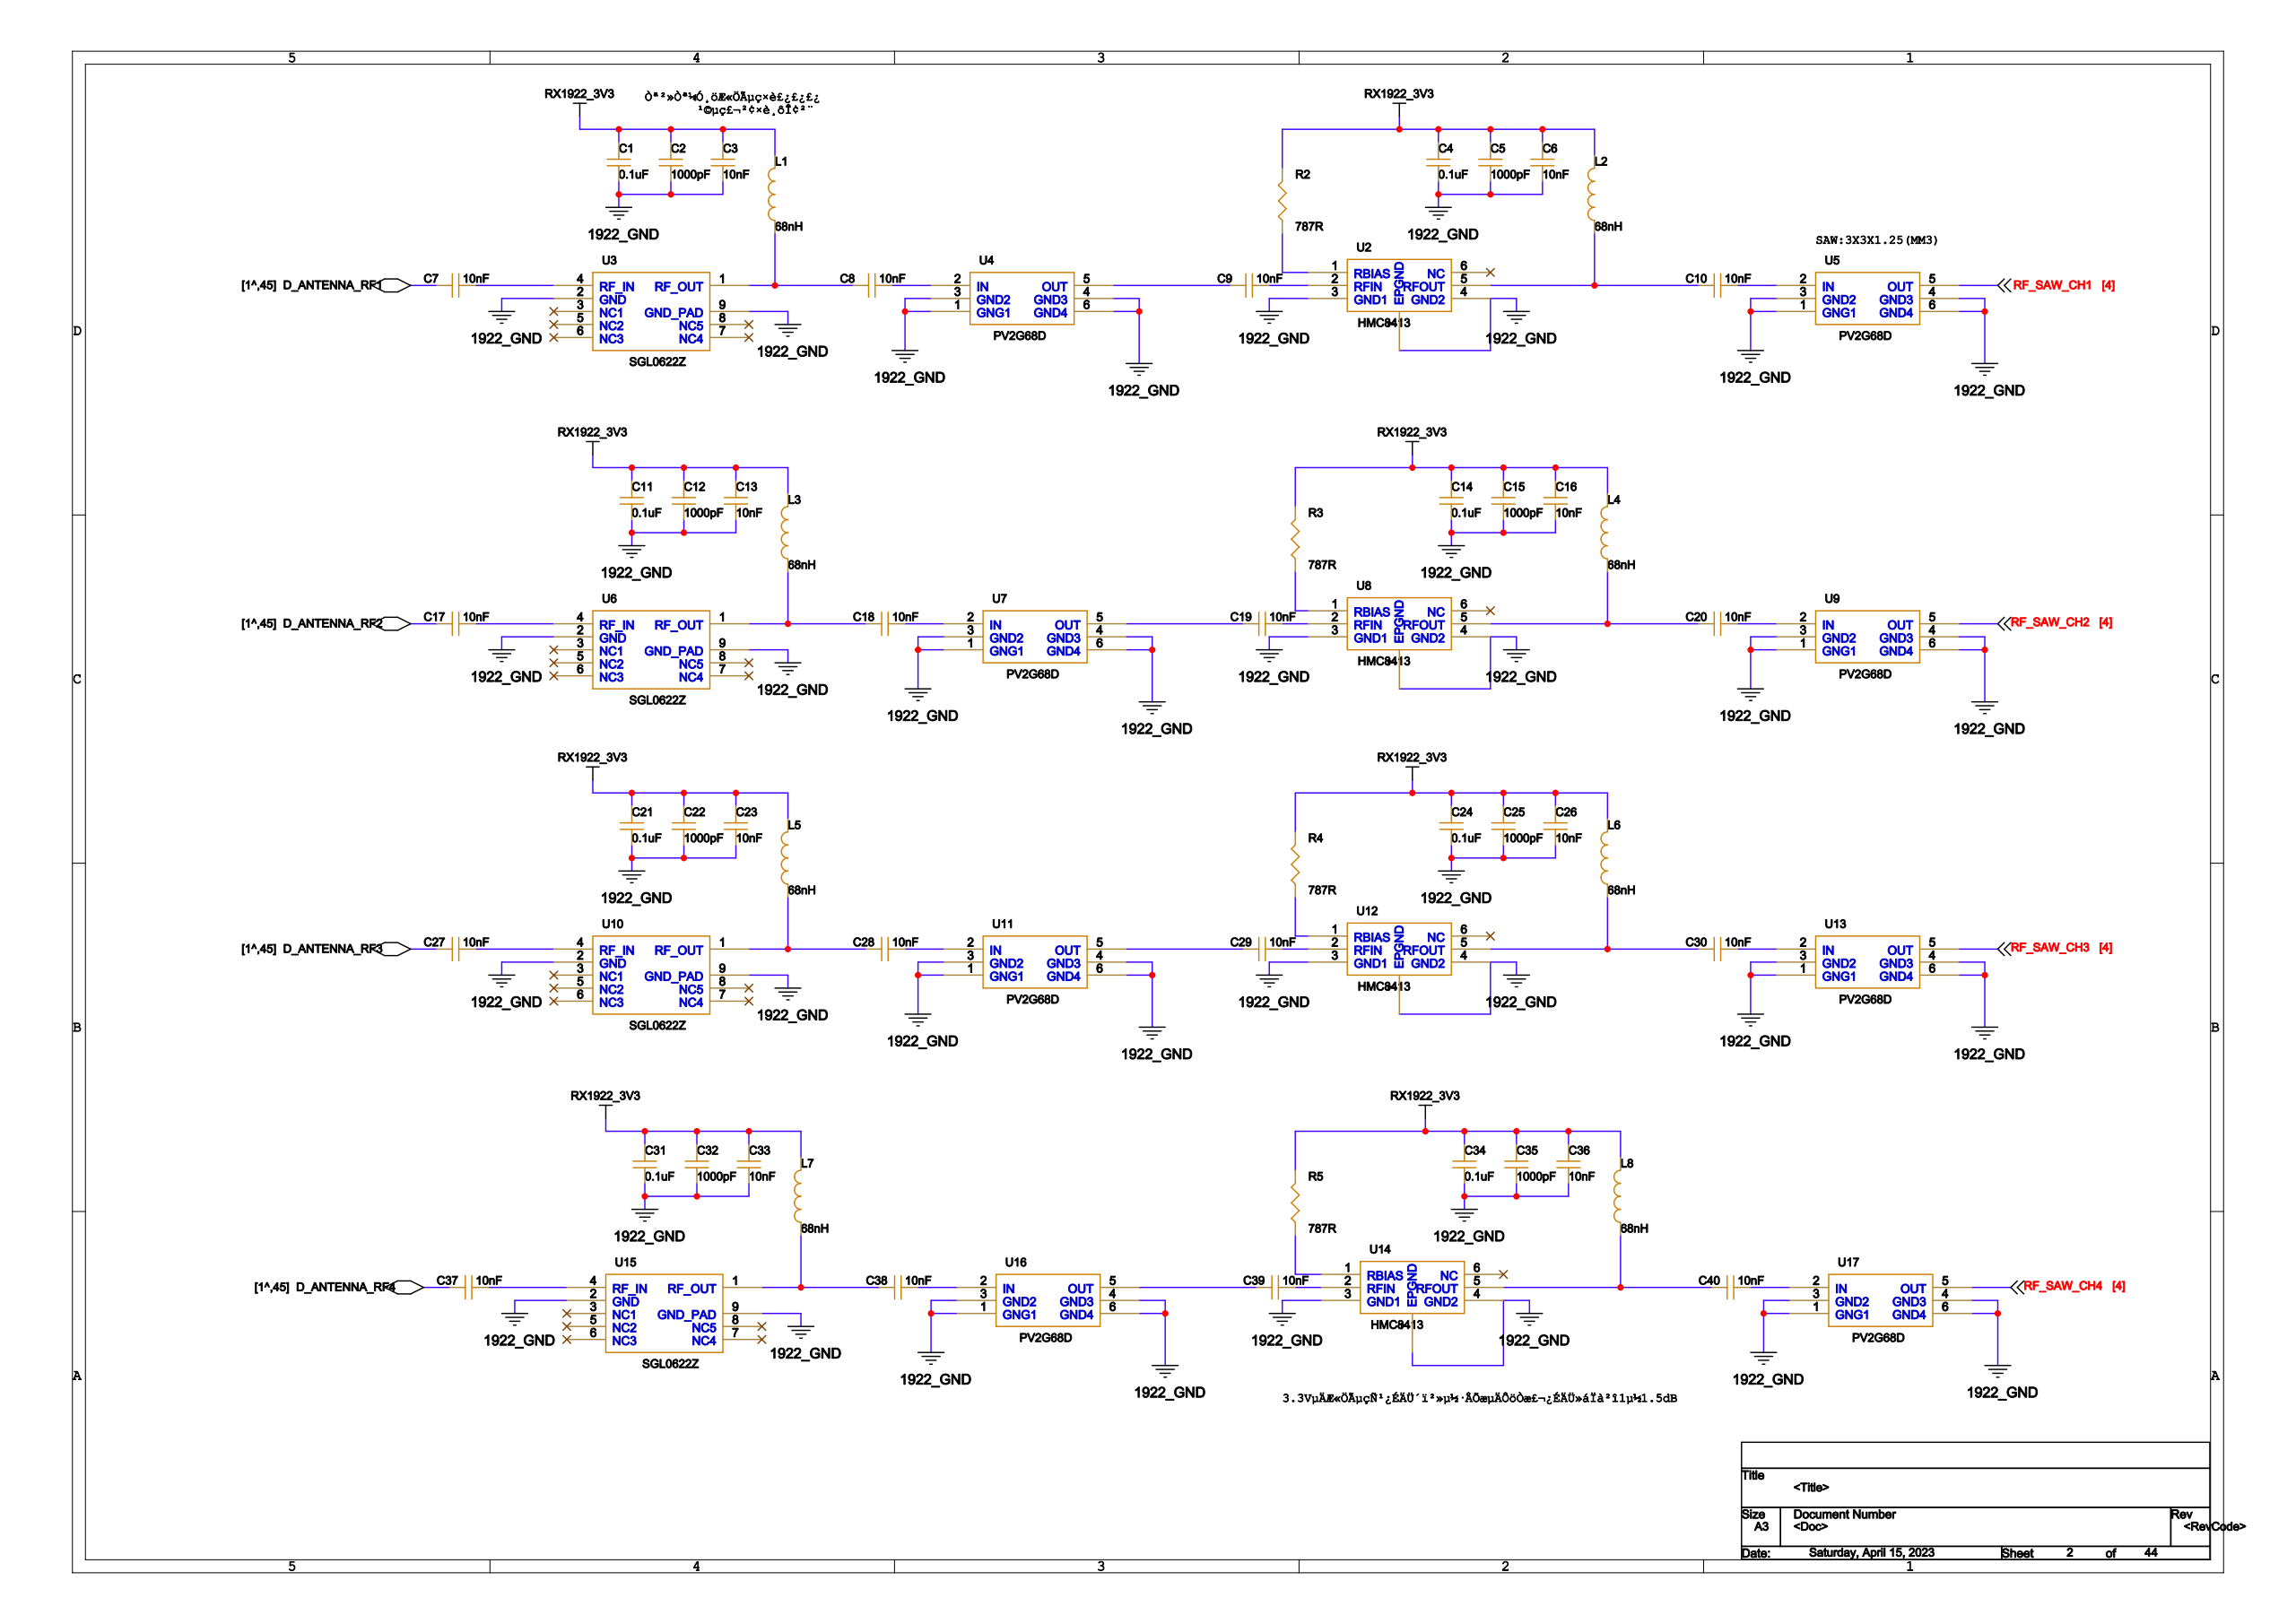Circuit board | Cadence Allegro | 1034 parts | 912 nets | one sheet of the schematic
Parts on this sheet (reference | value | footprint):
C1 | 0.1uF | C0402
C2 | 1000pF | C0402
C3 | 10nF | C0402
C4 | 0.1uF | C0402
C5 | 1000pF | C0402
C6 | 10nF | C0402
C7 | 10nF | C0402
C8 | 10nF | C0402
C9 | 10nF | C0402
C10 | 10nF | C0402
C11 | 0.1uF | C0402
C12 | 1000pF | C0402
C13 | 10nF | C0402
C14 | 0.1uF | C0402
C15 | 1000pF | C0402
C16 | 10nF | C0402
C17 | 10nF | C0402
C18 | 10nF | C0402
C19 | 10nF | C0402
C20 | 10nF | C0402
C21 | 0.1uF | C0402
C22 | 1000pF | C0402
C23 | 10nF | C0402
C24 | 0.1uF | C0402
C25 | 1000pF | C0402
C26 | 10nF | C0402
C27 | 10nF | C0402
C28 | 10nF | C0402
C29 | 10nF | C0402
C30 | 10nF | C0402
C31 | 0.1uF | C0402
C32 | 1000pF | C0402
C33 | 10nF | C0402
C34 | 0.1uF | C0402
C35 | 1000pF | C0402
C36 | 10nF | C0402
C37 | 10nF | C0402
C38 | 10nF | C0402
C39 | 10nF | C0402
C40 | 10nF | C0402
L1 | 68nH | L0402
L2 | 68nH | L0402
L3 | 68nH | L0402
L4 | 68nH | L0402
L5 | 68nH | L0402
L6 | 68nH | L0402
L7 | 68nH | L0402
L8 | 68nH | L0402
R2 | 787R | R0402
R3 | 787R | R0402
R4 | 787R | R0402
R5 | 787R | R0402
U2 | HMC8413 | HMC8413_LFCSP
U3 | SGL0622Z | GL0622_DFN
U4 | PV2G68D | G68D_DCC6C
U5 | PV2G68D | G68D_DCC6C
U6 | SGL0622Z | GL0622_DFN
U7 | PV2G68D | G68D_DCC6C
U8 | HMC8413 | HMC8413_LFCSP
U9 | PV2G68D | G68D_DCC6C
U10 | SGL0622Z | GL0622_DFN
U11 | PV2G68D | G68D_DCC6C
U12 | HMC8413 | HMC8413_LFCSP
U13 | PV2G68D | G68D_DCC6C
U14 | HMC8413 | HMC8413_LFCSP
U15 | SGL0622Z | GL0622_DFN
U16 | PV2G68D | G68D_DCC6C
U17 | PV2G68D | G68D_DCC6C
Nets of these parts (net: part-pin ...):
RF_SAW_CH1_D1: U5-5
RF_SAW_CH2_D1: U9-5
RF_SAW_CH3_D1: U13-5
RF_SAW_CH4_D1: U17-5
1922_GND: C1-1 C2-1 C3-1 C4-1 C5-1 C6-1 C11-1 C12-1 C13-1 C14-1 C15-1 C16-1 C21-1 C22-1 C23-1 C24-1 C25-1 C26-1 C31-1 C32-1 C33-1 C34-1 C35-1 C36-1 U2-3 U2-4 U2-7 U3-2 U3-9 U4-1 U4-3 U4-4 U4-6 U5-1 U5-3 U5-4 U5-6 U6-2 U6-9 U7-1 U7-3 U7-4 U7-6 U8-3 U8-4 U8-7 U9-1 U9-3 U9-4 U9-6 U10-2 U10-9 U11-1 U11-3 U11-4 U11-6 U12-3 U12-4 U12-7 U13-1 U13-3 U13-4 U13-6 U14-3 U14-4 U14-7 U15-2 U15-9 U16-1 U16-3 U16-4 U16-6 U17-1 U17-3 U17-4 U17-6
PWR1922_3V3_1: C1-2 C2-2 C3-2 C4-2 C5-2 C6-2 C11-2 C12-2 C13-2 C14-2 C15-2 C16-2 C21-2 C22-2 C23-2 C24-2 C25-2 C26-2 C31-2 C32-2 C33-2 C34-2 C35-2 C36-2 L1-2 L2-2 L3-2 L4-2 L5-2 L6-2 L7-2 L8-2 R2-2 R3-2 R4-2 R5-2
N14181388_D1: R4-1 U12-1
N14161069_D1: C29-2 U12-2
N14158707_D1: C30-1 L6-1 U12-5
N14181679_D1: R5-1 U14-1
N14161133_D1: C39-2 U14-2
N14159525_D1: C40-1 L8-1 U14-5
N14178364_D1: R2-1 U2-1
N14160942_D1: C9-2 U2-2
N14157205_D1: C10-1 L2-1 U2-5
N14181093_D1: R3-1 U8-1
N14161005_D1: C19-2 U8-2
N14157931_D1: C20-1 L4-1 U8-5
N14088748_D1: C10-2 U5-2
N244684: C17-1
N14091229_D1: C17-2 U6-4
N14147816_D1: C18-1 L3-1 U6-1
N14166037_D1: C18-2 U7-2
N14166041_D1: C19-1 U7-5
N14089401_D1: C20-2 U9-2
N244688: C27-1
N14091629_D1: C27-2 U10-4
N14147828_D1: C28-1 L5-1 U10-1
N14166455_D1: C28-2 U11-2
N14166459_D1: C29-1 U11-5
N14089671_D1: C30-2 U13-2
N244692: C37-1
N14092049_D1: C37-2 U15-4
N14147820_D1: C38-1 L7-1 U15-1
N14166887_D1: C38-2 U16-2
N14166891_D1: C39-1 U16-5
N14089951_D1: C40-2 U17-2
N244680: C7-1
N14090512_D1: C7-2 U3-4
N14147824_D1: C8-1 L1-1 U3-1
N14165389_D1: C8-2 U4-2
N14165393_D1: C9-1 U4-5